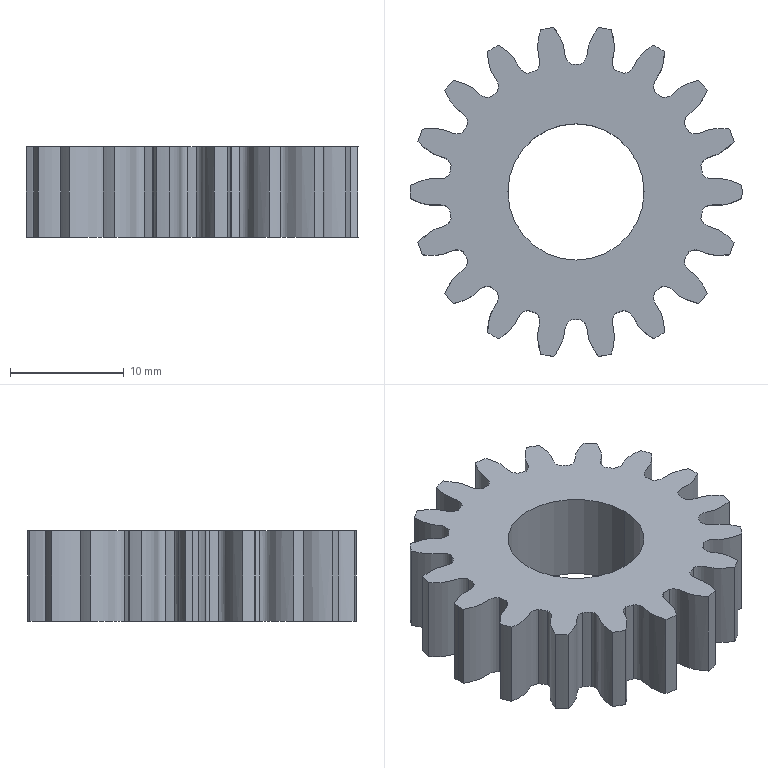Part | SolidWorks | features CirPattern 1, Cut 1, Extrusion 1, ICE 1, RefAxis 1 | 1 solid | 77 faces | box 29.25 x 28.982 x 8 mm | volume 3303 mm3 | cylinder 39 | spline 36 | plane 2 | commonest cylinder face diameters 29.25 x19 22.5 x18 12 x2